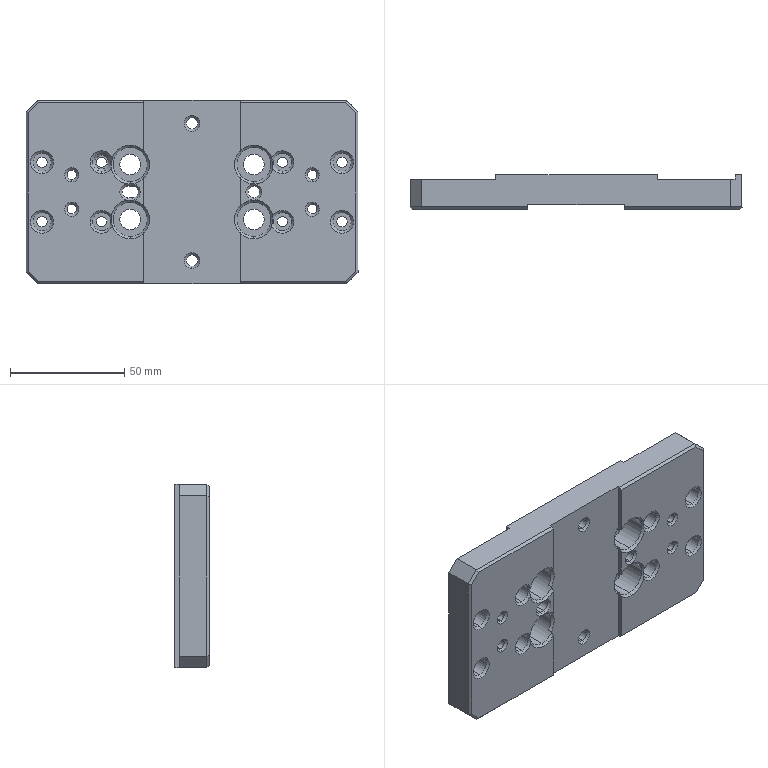Part | SolidWorks | features BaseBody 1 | 1 solid | 178 faces | box 145 x 15 x 80 mm | volume 139188 mm3 | cylinder 68 | cone 58 | plane 52 | commonest cylinder face diameters 4.5 x16 8 x16 4.2 x8 5 x8 9 x8 15 x8